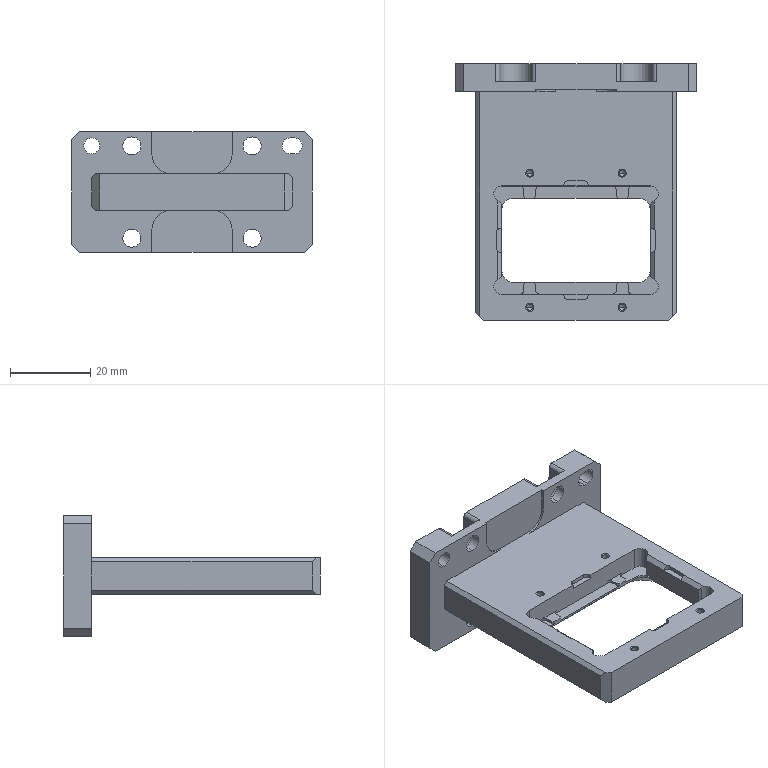NC program | NX | posted with a generic post | part box 60 x 64 x 30 mm
Whole program, first 2291 of 2766 lines:
N10 G17 G21 G94 G90
(FLOOR_WALL_COPY , TOOL : D20R0.8)
N12 T01 M6
N14 G54
N16 G17 G0 G90 X45. Y-29.999 B0. C0. S7500 M3
N18 G43 Z30. H1
N20 Z3.
N22 G94 G1 Z0. F1350.
N24 X42.
N26 X-42.
N28 Y-25.922
N30 Y-21.226
N32 X42.
N34 Y-12.453
N36 X-42.
N38 Y-3.68
N40 X42.
N42 Y5.094
N44 X-42.
N46 Y13.867
N48 X42.
N50 Y22.64
N52 X-42.
N54 X-45.
N56 Z3.
N58 G0 Z30.
N60 M5
(FLOOR_WALL_1_COPY_1 , TOOL : D10)
N62 T10 M6
N64 G54
N66 G17 G0 G90 X39.5 Y1.443 B0. C0. S9500 M3
N68 G43 Z30. H10
N70 Z1.153
N72 G94 G1 Z-0.347 F1000.
N74 X38.5 Y0.866
N76 G3 X38. Y0. R1.
N78 G1 Y-25.485 F3000.
N80 X33.485 Y-30.
N82 X-19.9
N84 Y-0.895
N86 X-20.4
N88 Y0.895
N90 X-19.9
N92 Y30.
N94 X33.485
N96 X38. Y25.485
N98 Y0.
N100 X32.
N102 Y-23.
N104 X31. Y-24.
N106 X-13.9
N108 Y-0.895
N110 G3 X-13.967 Y0. R6.
N112 X-13.9 Y0.895 R6.
N114 G1 Y24.
N116 X31.
N118 X32. Y23.
N120 Y0.
N122 X26.
N124 Y-18.
N126 X-7.9
N128 Y-0.895
N130 G3 X-7.933 Y0. R12.
N132 X-7.9 Y0.895 R12.
N134 G1 Y18.
N136 X26.
N138 Y0.
N140 X20.
N142 Y-12.
N144 X-1.9
N146 Y-0.895
N148 G3 X-1.922 Y0. R18.
N150 X-1.9 Y0.895 R18.
N152 G1 Y12.
N154 X20.
N156 Y0.
N158 X14.
N160 Y-6.
N162 X4.1
N164 Y-0.895
N166 G3 X4.083 Y0. R24.
N168 X4.1 Y0.895 R24.
N170 G1 Y6.
N172 X14.
N174 Y0.
N176 X9.5
N178 Y-1.5
N180 X8.6
N182 Y-0.895
N184 G3 X8.586 Y0. R28.5
N186 X8.6 Y0.895 R28.5
N188 G1 Y1.5
N190 X9.5
N192 Y0.
N194 G3 X10. Y-0.866 R1.
N196 G1 Z1.153
N198 G0 X39.5 Y1.443 Z0.807
N200 G1 Z-0.693 F1000.
N202 X38.5 Y0.866
N204 G3 X38. Y0. R1.
N206 G1 Y-25.485 F3000.
N208 X33.485 Y-30.
N210 X-19.9
N212 Y-0.895
N214 X-20.4
N216 Y0.895
N218 X-19.9
N220 Y30.
N222 X33.485
N224 X38. Y25.485
N226 Y0.
N228 X32.
N230 Y-23.
N232 X31. Y-24.
N234 X-13.9
N236 Y-0.895
N238 G3 X-13.967 Y0. R6.
N240 X-13.9 Y0.895 R6.
N242 G1 Y24.
N244 X31.
N246 X32. Y23.
N248 Y0.
N250 X26.
N252 Y-18.
N254 X-7.9
N256 Y-0.895
N258 G3 X-7.933 Y0. R12.
N260 X-7.9 Y0.895 R12.
N262 G1 Y18.
N264 X26.
N266 Y0.
N268 X20.
N270 Y-12.
N272 X-1.9
N274 Y-0.895
N276 G3 X-1.922 Y0. R18.
N278 X-1.9 Y0.895 R18.
N280 G1 Y12.
N282 X20.
N284 Y0.
N286 X14.
N288 Y-6.
N290 X4.1
N292 Y-0.895
N294 G3 X4.083 Y0. R24.
N296 X4.1 Y0.895 R24.
N298 G1 Y6.
N300 X14.
N302 Y0.
N304 X9.5
N306 Y-1.5
N308 X8.6
N310 Y-0.895
N312 G3 X8.586 Y0. R28.5
N314 X8.6 Y0.895 R28.5
N316 G1 Y1.5
N318 X9.5
N320 Y0.
N322 G3 X10. Y-0.866 R1.
N324 G1 Z0.807
N326 G0 X39.5 Y1.443 Z0.46
N328 G1 Z-1.04 F1000.
N330 X38.5 Y0.866
N332 G3 X38. Y0. R1.
N334 G1 Y-25.485 F3000.
N336 X33.485 Y-30.
N338 X-19.9
N340 Y-0.895
N342 X-20.4
N344 Y0.895
N346 X-19.9
N348 Y30.
N350 X33.485
N352 X38. Y25.485
N354 Y0.
N356 X32.
N358 Y-23.
N360 X31. Y-24.
N362 X-13.9
N364 Y-0.895
N366 G3 X-13.967 Y0. R6.
N368 X-13.9 Y0.895 R6.
N370 G1 Y24.
N372 X31.
N374 X32. Y23.
N376 Y0.
N378 X26.
N380 Y-18.
N382 X-7.9
N384 Y-0.895
N386 G3 X-7.933 Y0. R12.
N388 X-7.9 Y0.895 R12.
N390 G1 Y18.
N392 X26.
N394 Y0.
N396 X20.
N398 Y-12.
N400 X-1.9
N402 Y-0.895
N404 G3 X-1.922 Y0. R18.
N406 X-1.9 Y0.895 R18.
N408 G1 Y12.
N410 X20.
N412 Y0.
N414 X14.
N416 Y-6.
N418 X4.1
N420 Y-0.895
N422 G3 X4.083 Y0. R24.
N424 X4.1 Y0.895 R24.
N426 G1 Y6.
N428 X14.
N430 Y0.
N432 X9.5
N434 Y-1.5
N436 X8.6
N438 Y-0.895
N440 G3 X8.586 Y0. R28.5
N442 X8.6 Y0.895 R28.5
N444 G1 Y1.5
N446 X9.5
N448 Y0.
N450 G3 X10. Y-0.866 R1.
N452 G1 Z0.46
N454 G0 X39.5 Y1.443 Z0.113
N456 G1 Z-1.387 F1000.
N458 X38.5 Y0.866
N460 G3 X38. Y0. R1.
N462 G1 Y-25.485 F3000.
N464 X33.485 Y-30.
N466 X-19.9
N468 Y-0.895
N470 X-20.4
N472 Y0.895
N474 X-19.9
N476 Y30.
N478 X33.485
N480 X38. Y25.485
N482 Y0.
N484 X32.
N486 Y-23.
N488 X31. Y-24.
N490 X-13.9
N492 Y-0.895
N494 G3 X-13.967 Y0. R6.
N496 X-13.9 Y0.895 R6.
N498 G1 Y24.
N500 X31.
N502 X32. Y23.
N504 Y0.
N506 X26.
N508 Y-18.
N510 X-7.9
N512 Y-0.895
N514 G3 X-7.933 Y0. R12.
N516 X-7.9 Y0.895 R12.
N518 G1 Y18.
N520 X26.
N522 Y0.
N524 X20.
N526 Y-12.
N528 X-1.9
N530 Y-0.895
N532 G3 X-1.922 Y0. R18.
N534 X-1.9 Y0.895 R18.
N536 G1 Y12.
N538 X20.
N540 Y0.
N542 X14.
N544 Y-6.
N546 X4.1
N548 Y-0.895
N550 G3 X4.083 Y0. R24.
N552 X4.1 Y0.895 R24.
N554 G1 Y6.
N556 X14.
N558 Y0.
N560 X9.5
N562 Y-1.5
N564 X8.6
N566 Y-0.895
N568 G3 X8.586 Y0. R28.5
N570 X8.6 Y0.895 R28.5
N572 G1 Y1.5
N574 X9.5
N576 Y0.
N578 G3 X10. Y-0.866 R1.
N580 G1 Z0.113
N582 G0 X39.5 Y1.443 Z-0.233
N584 G1 Z-1.733 F1000.
N586 X38.5 Y0.866
N588 G3 X38. Y0. R1.
N590 G1 Y-25.485 F3000.
N592 X33.485 Y-30.
N594 X-19.9
N596 Y-0.895
N598 X-20.4
N600 Y0.895
N602 X-19.9
N604 Y30.
N606 X33.485
N608 X38. Y25.485
N610 Y0.
N612 X32.
N614 Y-23.
N616 X31. Y-24.
N618 X-13.9
N620 Y-0.895
N622 G3 X-13.967 Y0. R6.
N624 X-13.9 Y0.895 R6.
N626 G1 Y24.
N628 X31.
N630 X32. Y23.
N632 Y0.
N634 X26.
N636 Y-18.
N638 X-7.9
N640 Y-0.895
N642 G3 X-7.933 Y0. R12.
N644 X-7.9 Y0.895 R12.
N646 G1 Y18.
N648 X26.
N650 Y0.
N652 X20.
N654 Y-12.
N656 X-1.9
N658 Y-0.895
N660 G3 X-1.922 Y0. R18.
N662 X-1.9 Y0.895 R18.
N664 G1 Y12.
N666 X20.
N668 Y0.
N670 X14.
N672 Y-6.
N674 X4.1
N676 Y-0.895
N678 G3 X4.083 Y0. R24.
N680 X4.1 Y0.895 R24.
N682 G1 Y6.
N684 X14.
N686 Y0.
N688 X9.5
N690 Y-1.5
N692 X8.6
N694 Y-0.895
N696 G3 X8.586 Y0. R28.5
N698 X8.6 Y0.895 R28.5
N700 G1 Y1.5
N702 X9.5
N704 Y0.
N706 G3 X10. Y-0.866 R1.
N708 G1 Z-0.233
N710 G0 X39.5 Y1.443 Z-0.58
N712 G1 Z-2.08 F1000.
N714 X38.5 Y0.866
N716 G3 X38. Y0. R1.
N718 G1 Y-25.485 F3000.
N720 X33.485 Y-30.
N722 X-19.9
N724 Y-0.895
N726 X-20.4
N728 Y0.895
N730 X-19.9
N732 Y30.
N734 X33.485
N736 X38. Y25.485
N738 Y0.
N740 X32.
N742 Y-23.
N744 X31. Y-24.
N746 X-13.9
N748 Y-0.895
N750 G3 X-13.967 Y0. R6.
N752 X-13.9 Y0.895 R6.
N754 G1 Y24.
N756 X31.
N758 X32. Y23.
N760 Y0.
N762 X26.
N764 Y-18.
N766 X-7.9
N768 Y-0.895
N770 G3 X-7.933 Y0. R12.
N772 X-7.9 Y0.895 R12.
N774 G1 Y18.
N776 X26.
N778 Y0.
N780 X20.
N782 Y-12.
N784 X-1.9
N786 Y-0.895
N788 G3 X-1.922 Y0. R18.
N790 X-1.9 Y0.895 R18.
N792 G1 Y12.
N794 X20.
N796 Y0.
N798 X14.
N800 Y-6.
N802 X4.1
N804 Y-0.895
N806 G3 X4.083 Y0. R24.
N808 X4.1 Y0.895 R24.
N810 G1 Y6.
N812 X14.
N814 Y0.
N816 X9.5
N818 Y-1.5
N820 X8.6
N822 Y-0.895
N824 G3 X8.586 Y0. R28.5
N826 X8.6 Y0.895 R28.5
N828 G1 Y1.5
N830 X9.5
N832 Y0.
N834 G3 X10. Y-0.866 R1.
N836 G1 Z-0.58
N838 G0 X39.5 Y1.443 Z-0.927
N840 G1 Z-2.427 F1000.
N842 X38.5 Y0.866
N844 G3 X38. Y0. R1.
N846 G1 Y-25.485 F3000.
N848 X33.485 Y-30.
N850 X-19.9
N852 Y-0.895
N854 X-20.4
N856 Y0.895
N858 X-19.9
N860 Y30.
N862 X33.485
N864 X38. Y25.485
N866 Y0.
N868 X32.
N870 Y-23.
N872 X31. Y-24.
N874 X-13.9
N876 Y-0.895
N878 G3 X-13.967 Y0. R6.
N880 X-13.9 Y0.895 R6.
N882 G1 Y24.
N884 X31.
N886 X32. Y23.
N888 Y0.
N890 X26.
N892 Y-18.
N894 X-7.9
N896 Y-0.895
N898 G3 X-7.933 Y0. R12.
N900 X-7.9 Y0.895 R12.
N902 G1 Y18.
N904 X26.
N906 Y0.
N908 X20.
N910 Y-12.
N912 X-1.9
N914 Y-0.895
N916 G3 X-1.922 Y0. R18.
N918 X-1.9 Y0.895 R18.
N920 G1 Y12.
N922 X20.
N924 Y0.
N926 X14.
N928 Y-6.
N930 X4.1
N932 Y-0.895
N934 G3 X4.083 Y0. R24.
N936 X4.1 Y0.895 R24.
N938 G1 Y6.
N940 X14.
N942 Y0.
N944 X9.5
N946 Y-1.5
N948 X8.6
N950 Y-0.895
N952 G3 X8.586 Y0. R28.5
N954 X8.6 Y0.895 R28.5
N956 G1 Y1.5
N958 X9.5
N960 Y0.
N962 G3 X10. Y-0.866 R1.
N964 G1 Z-0.927
N966 G0 X39.5 Y1.443 Z-1.273
N968 G1 Z-2.773 F1000.
N970 X38.5 Y0.866
N972 G3 X38. Y0. R1.
N974 G1 Y-25.485 F3000.
N976 X33.485 Y-30.
N978 X-19.9
N980 Y-0.895
N982 X-20.4
N984 Y0.895
N986 X-19.9
N988 Y30.
N990 X33.485
N992 X38. Y25.485
N994 Y0.
N996 X32.
N998 Y-23.
N1000 X31. Y-24.
N1002 X-13.9
N1004 Y-0.895
N1006 G3 X-13.967 Y0. R6.
N1008 X-13.9 Y0.895 R6.
N1010 G1 Y24.
N1012 X31.
N1014 X32. Y23.
N1016 Y0.
N1018 X26.
N1020 Y-18.
N1022 X-7.9
N1024 Y-0.895
N1026 G3 X-7.933 Y0. R12.
N1028 X-7.9 Y0.895 R12.
N1030 G1 Y18.
N1032 X26.
N1034 Y0.
N1036 X20.
N1038 Y-12.
N1040 X-1.9
N1042 Y-0.895
N1044 G3 X-1.922 Y0. R18.
N1046 X-1.9 Y0.895 R18.
N1048 G1 Y12.
N1050 X20.
N1052 Y0.
N1054 X14.
N1056 Y-6.
N1058 X4.1
N1060 Y-0.895
N1062 G3 X4.083 Y0. R24.
N1064 X4.1 Y0.895 R24.
N1066 G1 Y6.
N1068 X14.
N1070 Y0.
N1072 X9.5
N1074 Y-1.5
N1076 X8.6
N1078 Y-0.895
N1080 G3 X8.586 Y0. R28.5
N1082 X8.6 Y0.895 R28.5
N1084 G1 Y1.5
N1086 X9.5
N1088 Y0.
N1090 G3 X10. Y-0.866 R1.
N1092 G1 Z-1.273
N1094 G0 X39.5 Y1.443 Z-1.62
N1096 G1 Z-3.12 F1000.
N1098 X38.5 Y0.866
N1100 G3 X38. Y0. R1.
N1102 G1 Y-25.485 F3000.
N1104 X33.485 Y-30.
N1106 X-19.9
N1108 Y-0.895
N1110 X-20.4
N1112 Y0.895
N1114 X-19.9
N1116 Y30.
N1118 X33.485
N1120 X38. Y25.485
N1122 Y0.
N1124 X32.
N1126 Y-23.
N1128 X31. Y-24.
N1130 X-13.9
N1132 Y-0.895
N1134 G3 X-13.967 Y0. R6.
N1136 X-13.9 Y0.895 R6.
N1138 G1 Y24.
N1140 X31.
N1142 X32. Y23.
N1144 Y0.
N1146 X26.
N1148 Y-18.
N1150 X-7.9
N1152 Y-0.895
N1154 G3 X-7.933 Y0. R12.
N1156 X-7.9 Y0.895 R12.
N1158 G1 Y18.
N1160 X26.
N1162 Y0.
N1164 X20.
N1166 Y-12.
N1168 X-1.9
N1170 Y-0.895
N1172 G3 X-1.922 Y0. R18.
N1174 X-1.9 Y0.895 R18.
N1176 G1 Y12.
N1178 X20.
N1180 Y0.
N1182 X14.
N1184 Y-6.
N1186 X4.1
N1188 Y-0.895
N1190 G3 X4.083 Y0. R24.
N1192 X4.1 Y0.895 R24.
N1194 G1 Y6.
N1196 X14.
N1198 Y0.
N1200 X9.5
N1202 Y-1.5
N1204 X8.6
N1206 Y-0.895
N1208 G3 X8.586 Y0. R28.5
N1210 X8.6 Y0.895 R28.5
N1212 G1 Y1.5
N1214 X9.5
N1216 Y0.
N1218 G3 X10. Y-0.866 R1.
N1220 G1 Z-1.62
N1222 G0 X39.5 Y1.443 Z-1.967
N1224 G1 Z-3.467 F1000.
N1226 X38.5 Y0.866
N1228 G3 X38. Y0. R1.
N1230 G1 Y-25.485 F3000.
N1232 X33.485 Y-30.
N1234 X-19.9
N1236 Y-0.895
N1238 X-20.4
N1240 Y0.895
N1242 X-19.9
N1244 Y30.
N1246 X33.485
N1248 X38. Y25.485
N1250 Y0.
N1252 X32.
N1254 Y-23.
N1256 X31. Y-24.
N1258 X-13.9
N1260 Y-0.895
N1262 G3 X-13.967 Y0. R6.
N1264 X-13.9 Y0.895 R6.
N1266 G1 Y24.
N1268 X31.
N1270 X32. Y23.
N1272 Y0.
N1274 X26.
N1276 Y-18.
N1278 X-7.9
N1280 Y-0.895
N1282 G3 X-7.933 Y0. R12.
N1284 X-7.9 Y0.895 R12.
N1286 G1 Y18.
N1288 X26.
N1290 Y0.
N1292 X20.
N1294 Y-12.
N1296 X-1.9
N1298 Y-0.895
N1300 G3 X-1.922 Y0. R18.
N1302 X-1.9 Y0.895 R18.
N1304 G1 Y12.
N1306 X20.
N1308 Y0.
N1310 X14.
N1312 Y-6.
N1314 X4.1
N1316 Y-0.895
N1318 G3 X4.083 Y0. R24.
N1320 X4.1 Y0.895 R24.
N1322 G1 Y6.
N1324 X14.
N1326 Y0.
N1328 X9.5
N1330 Y-1.5
N1332 X8.6
N1334 Y-0.895
N1336 G3 X8.586 Y0. R28.5
N1338 X8.6 Y0.895 R28.5
N1340 G1 Y1.5
N1342 X9.5
N1344 Y0.
N1346 G3 X10. Y-0.866 R1.
N1348 G1 Z-1.967
N1350 G0 X39.5 Y1.443 Z-2.313
N1352 G1 Z-3.813 F1000.
N1354 X38.5 Y0.866
N1356 G3 X38. Y0. R1.
N1358 G1 Y-25.485 F3000.
N1360 X33.485 Y-30.
N1362 X-19.9
N1364 Y-0.895
N1366 X-20.4
N1368 Y0.895
N1370 X-19.9
N1372 Y30.
N1374 X33.485
N1376 X38. Y25.485
N1378 Y0.
N1380 X32.
N1382 Y-23.
N1384 X31. Y-24.
N1386 X-13.9
N1388 Y-0.895
N1390 G3 X-13.967 Y0. R6.
N1392 X-13.9 Y0.895 R6.
N1394 G1 Y24.
N1396 X31.
N1398 X32. Y23.
N1400 Y0.
N1402 X26.
N1404 Y-18.
N1406 X-7.9
N1408 Y-0.895
N1410 G3 X-7.933 Y0. R12.
N1412 X-7.9 Y0.895 R12.
N1414 G1 Y18.
N1416 X26.
N1418 Y0.
N1420 X20.
N1422 Y-12.
N1424 X-1.9
N1426 Y-0.895
N1428 G3 X-1.922 Y0. R18.
N1430 X-1.9 Y0.895 R18.
N1432 G1 Y12.
N1434 X20.
N1436 Y0.
N1438 X14.
N1440 Y-6.
N1442 X4.1
N1444 Y-0.895
N1446 G3 X4.083 Y0. R24.
N1448 X4.1 Y0.895 R24.
N1450 G1 Y6.
N1452 X14.
N1454 Y0.
N1456 X9.5
N1458 Y-1.5
N1460 X8.6
N1462 Y-0.895
N1464 G3 X8.586 Y0. R28.5
N1466 X8.6 Y0.895 R28.5
N1468 G1 Y1.5
N1470 X9.5
N1472 Y0.
N1474 G3 X10. Y-0.866 R1.
N1476 G1 Z-2.313
N1478 G0 X39.5 Y1.443 Z-2.66
N1480 G1 Z-4.16 F1000.
N1482 X38.5 Y0.866
N1484 G3 X38. Y0. R1.
N1486 G1 Y-25.485 F3000.
N1488 X33.485 Y-30.
N1490 X-19.9
N1492 Y-0.895
N1494 X-20.4
N1496 Y0.895
N1498 X-19.9
N1500 Y30.
N1502 X33.485
N1504 X38. Y25.485
N1506 Y0.
N1508 X32.
N1510 Y-23.
N1512 X31. Y-24.
N1514 X-13.9
N1516 Y-0.895
N1518 G3 X-13.967 Y0. R6.
N1520 X-13.9 Y0.895 R6.
N1522 G1 Y24.
N1524 X31.
N1526 X32. Y23.
N1528 Y0.
N1530 X26.
N1532 Y-18.
N1534 X-7.9
N1536 Y-0.895
N1538 G3 X-7.933 Y0. R12.
N1540 X-7.9 Y0.895 R12.
N1542 G1 Y18.
N1544 X26.
N1546 Y0.
N1548 X20.
N1550 Y-12.
N1552 X-1.9
N1554 Y-0.895
N1556 G3 X-1.922 Y0. R18.
N1558 X-1.9 Y0.895 R18.
N1560 G1 Y12.
N1562 X20.
N1564 Y0.
N1566 X14.
N1568 Y-6.
N1570 X4.1
N1572 Y-0.895
N1574 G3 X4.083 Y0. R24.
N1576 X4.1 Y0.895 R24.
N1578 G1 Y6.
N1580 X14.
N1582 Y0.
N1584 X9.5
N1586 Y-1.5
N1588 X8.6
N1590 Y-0.895
N1592 G3 X8.586 Y0. R28.5
N1594 X8.6 Y0.895 R28.5
N1596 G1 Y1.5
N1598 X9.5
N1600 Y0.
N1602 G3 X10. Y-0.866 R1.
N1604 G1 Z-2.66
N1606 G0 X39.5 Y1.443 Z-3.007
N1608 G1 Z-4.507 F1000.
N1610 X38.5 Y0.866
N1612 G3 X38. Y0. R1.
N1614 G1 Y-25.485 F3000.
N1616 X33.485 Y-30.
N1618 X-19.9
N1620 Y-0.895
N1622 X-20.4
N1624 Y0.895
N1626 X-19.9
N1628 Y30.
N1630 X33.485
N1632 X38. Y25.485
N1634 Y0.
N1636 X32.
N1638 Y-23.
N1640 X31. Y-24.
N1642 X-13.9
N1644 Y-0.895
N1646 G3 X-13.967 Y0. R6.
N1648 X-13.9 Y0.895 R6.
N1650 G1 Y24.
N1652 X31.
N1654 X32. Y23.
N1656 Y0.
N1658 X26.
N1660 Y-18.
N1662 X-7.9
N1664 Y-0.895
N1666 G3 X-7.933 Y0. R12.
N1668 X-7.9 Y0.895 R12.
N1670 G1 Y18.
N1672 X26.
N1674 Y0.
N1676 X20.
N1678 Y-12.
N1680 X-1.9
N1682 Y-0.895
N1684 G3 X-1.922 Y0. R18.
N1686 X-1.9 Y0.895 R18.
N1688 G1 Y12.
N1690 X20.
N1692 Y0.
N1694 X14.
N1696 Y-6.
N1698 X4.1
N1700 Y-0.895
N1702 G3 X4.083 Y0. R24.
N1704 X4.1 Y0.895 R24.
N1706 G1 Y6.
N1708 X14.
N1710 Y0.
N1712 X9.5
N1714 Y-1.5
N1716 X8.6
N1718 Y-0.895
N1720 G3 X8.586 Y0. R28.5
N1722 X8.6 Y0.895 R28.5
N1724 G1 Y1.5
N1726 X9.5
N1728 Y0.
N1730 G3 X10. Y-0.866 R1.
N1732 G1 Z-3.007
N1734 G0 X39.5 Y1.443 Z-3.353
N1736 G1 Z-4.853 F1000.
N1738 X38.5 Y0.866
N1740 G3 X38. Y0. R1.
N1742 G1 Y-25.485 F3000.
N1744 X33.485 Y-30.
N1746 X-19.9
N1748 Y-0.895
N1750 X-20.4
N1752 Y0.895
N1754 X-19.9
N1756 Y30.
N1758 X33.485
N1760 X38. Y25.485
N1762 Y0.
N1764 X32.
N1766 Y-23.
N1768 X31. Y-24.
N1770 X-13.9
N1772 Y-0.895
N1774 G3 X-13.967 Y0. R6.
N1776 X-13.9 Y0.895 R6.
N1778 G1 Y24.
N1780 X31.
N1782 X32. Y23.
N1784 Y0.
N1786 X26.
N1788 Y-18.
N1790 X-7.9
N1792 Y-0.895
N1794 G3 X-7.933 Y0. R12.
N1796 X-7.9 Y0.895 R12.
N1798 G1 Y18.
N1800 X26.
N1802 Y0.
N1804 X20.
N1806 Y-12.
N1808 X-1.9
N1810 Y-0.895
N1812 G3 X-1.922 Y0. R18.
N1814 X-1.9 Y0.895 R18.
N1816 G1 Y12.
N1818 X20.
N1820 Y0.
N1822 X14.
N1824 Y-6.
N1826 X4.1
N1828 Y-0.895
N1830 G3 X4.083 Y0. R24.
N1832 X4.1 Y0.895 R24.
N1834 G1 Y6.
N1836 X14.
N1838 Y0.
N1840 X9.5
N1842 Y-1.5
N1844 X8.6
N1846 Y-0.895
N1848 G3 X8.586 Y0. R28.5
N1850 X8.6 Y0.895 R28.5
N1852 G1 Y1.5
N1854 X9.5
N1856 Y0.
N1858 G3 X10. Y-0.866 R1.
N1860 G1 Z-3.353
N1862 G0 X39.5 Y1.443 Z-3.7
N1864 G1 Z-5.2 F1000.
N1866 X38.5 Y0.866
N1868 G3 X38. Y0. R1.
N1870 G1 Y-25.485 F3000.
N1872 X33.485 Y-30.
N1874 X-19.9
N1876 Y-0.895
N1878 X-20.4
N1880 Y0.895
N1882 X-19.9
N1884 Y30.
N1886 X33.485
N1888 X38. Y25.485
N1890 Y0.
N1892 X32.
N1894 Y-23.
N1896 X31. Y-24.
N1898 X-13.9
N1900 Y-0.895
N1902 G3 X-13.967 Y0. R6.
N1904 X-13.9 Y0.895 R6.
N1906 G1 Y24.
N1908 X31.
N1910 X32. Y23.
N1912 Y0.
N1914 X26.
N1916 Y-18.
N1918 X-7.9
N1920 Y-0.895
N1922 G3 X-7.933 Y0. R12.
N1924 X-7.9 Y0.895 R12.
N1926 G1 Y18.
N1928 X26.
N1930 Y0.
N1932 X20.
N1934 Y-12.
N1936 X-1.9
N1938 Y-0.895
N1940 G3 X-1.922 Y0. R18.
N1942 X-1.9 Y0.895 R18.
N1944 G1 Y12.
N1946 X20.
N1948 Y0.
N1950 X14.
N1952 Y-6.
N1954 X4.1
N1956 Y-0.895
N1958 G3 X4.083 Y0. R24.
N1960 X4.1 Y0.895 R24.
N1962 G1 Y6.
N1964 X14.
N1966 Y0.
N1968 X9.5
N1970 Y-1.5
N1972 X8.6
N1974 Y-0.895
N1976 G3 X8.586 Y0. R28.5
N1978 X8.6 Y0.895 R28.5
N1980 G1 Y1.5
N1982 X9.5
N1984 Y0.
N1986 G3 X10. Y-0.866 R1.
N1988 G1 Z-3.7
N1990 G0 X39.5 Y1.443 Z-4.047
N1992 G1 Z-5.547 F1000.
N1994 X38.5 Y0.866
N1996 G3 X38. Y0. R1.
N1998 G1 Y-25.485 F3000.
N2000 X33.485 Y-30.
N2002 X-19.9
N2004 Y-0.895
N2006 X-20.4
N2008 Y0.895
N2010 X-19.9
N2012 Y30.
N2014 X33.485
N2016 X38. Y25.485
N2018 Y0.
N2020 X32.
N2022 Y-23.
N2024 X31. Y-24.
N2026 X-13.9
N2028 Y-0.895
N2030 G3 X-13.967 Y0. R6.
N2032 X-13.9 Y0.895 R6.
N2034 G1 Y24.
N2036 X31.
N2038 X32. Y23.
N2040 Y0.
N2042 X26.
N2044 Y-18.
N2046 X-7.9
N2048 Y-0.895
N2050 G3 X-7.933 Y0. R12.
N2052 X-7.9 Y0.895 R12.
N2054 G1 Y18.
N2056 X26.
N2058 Y0.
N2060 X20.
N2062 Y-12.
N2064 X-1.9
N2066 Y-0.895
N2068 G3 X-1.922 Y0. R18.
N2070 X-1.9 Y0.895 R18.
N2072 G1 Y12.
N2074 X20.
N2076 Y0.
N2078 X14.
N2080 Y-6.
N2082 X4.1
N2084 Y-0.895
N2086 G3 X4.083 Y0. R24.
N2088 X4.1 Y0.895 R24.
N2090 G1 Y6.
N2092 X14.
N2094 Y0.
N2096 X9.5
N2098 Y-1.5
N2100 X8.6
N2102 Y-0.895
N2104 G3 X8.586 Y0. R28.5
N2106 X8.6 Y0.895 R28.5
N2108 G1 Y1.5
N2110 X9.5
N2112 Y0.
N2114 G3 X10. Y-0.866 R1.
N2116 G1 Z-4.047
N2118 G0 X39.5 Y1.443 Z-4.393
N2120 G1 Z-5.893 F1000.
N2122 X38.5 Y0.866
N2124 G3 X38. Y0. R1.
N2126 G1 Y-25.485 F3000.
N2128 X33.485 Y-30.
N2130 X-19.9
N2132 Y-0.895
N2134 X-20.4
N2136 Y0.895
N2138 X-19.9
N2140 Y30.
N2142 X33.485
N2144 X38. Y25.485
N2146 Y0.
N2148 X32.
N2150 Y-23.
N2152 X31. Y-24.
N2154 X-13.9
N2156 Y-0.895
N2158 G3 X-13.967 Y0. R6.
N2160 X-13.9 Y0.895 R6.
N2162 G1 Y24.
N2164 X31.
N2166 X32. Y23.
N2168 Y0.
N2170 X26.
N2172 Y-18.
N2174 X-7.9
N2176 Y-0.895
N2178 G3 X-7.933 Y0. R12.
N2180 X-7.9 Y0.895 R12.
N2182 G1 Y18.
N2184 X26.
N2186 Y0.
N2188 X20.
N2190 Y-12.
N2192 X-1.9
N2194 Y-0.895
N2196 G3 X-1.922 Y0. R18.
N2198 X-1.9 Y0.895 R18.
N2200 G1 Y12.
N2202 X20.
N2204 Y0.
N2206 X14.
N2208 Y-6.
N2210 X4.1
N2212 Y-0.895
N2214 G3 X4.083 Y0. R24.
N2216 X4.1 Y0.895 R24.
N2218 G1 Y6.
N2220 X14.
N2222 Y0.
N2224 X9.5
N2226 Y-1.5
N2228 X8.6
N2230 Y-0.895
N2232 G3 X8.586 Y0. R28.5
N2234 X8.6 Y0.895 R28.5
N2236 G1 Y1.5
N2238 X9.5
N2240 Y0.
N2242 G3 X10. Y-0.866 R1.
N2244 G1 Z-4.393
N2246 G0 X39.5 Y1.443 Z-4.74
N2248 G1 Z-6.24 F1000.
N2250 X38.5 Y0.866
N2252 G3 X38. Y0. R1.
N2254 G1 Y-25.485 F3000.
N2256 X33.485 Y-30.
N2258 X-19.9
N2260 Y-0.895
N2262 X-20.4
N2264 Y0.895
N2266 X-19.9
N2268 Y30.
N2270 X33.485
N2272 X38. Y25.485
N2274 Y0.
N2276 X32.
N2278 Y-23.
N2280 X31. Y-24.
N2282 X-13.9
N2284 Y-0.895
N2286 G3 X-13.967 Y0. R6.
N2288 X-13.9 Y0.895 R6.
N2290 G1 Y24.
N2292 X31.
N2294 X32. Y23.
N2296 Y0.
N2298 X26.
N2300 Y-18.
N2302 X-7.9
N2304 Y-0.895
N2306 G3 X-7.933 Y0. R12.
N2308 X-7.9 Y0.895 R12.
N2310 G1 Y18.
N2312 X26.
N2314 Y0.
N2316 X20.
N2318 Y-12.
N2320 X-1.9
N2322 Y-0.895
N2324 G3 X-1.922 Y0. R18.
N2326 X-1.9 Y0.895 R18.
N2328 G1 Y12.
N2330 X20.
N2332 Y0.
N2334 X14.
N2336 Y-6.
N2338 X4.1
N2340 Y-0.895
N2342 G3 X4.083 Y0. R24.
N2344 X4.1 Y0.895 R24.
N2346 G1 Y6.
N2348 X14.
N2350 Y0.
N2352 X9.5
N2354 Y-1.5
N2356 X8.6
N2358 Y-0.895
N2360 G3 X8.586 Y0. R28.5
N2362 X8.6 Y0.895 R28.5
N2364 G1 Y1.5
N2366 X9.5
N2368 Y0.
N2370 G3 X10. Y-0.866 R1.
N2372 G1 Z-4.74
N2374 G0 X39.5 Y1.443 Z-5.087
N2376 G1 Z-6.587 F1000.
N2378 X38.5 Y0.866
N2380 G3 X38. Y0. R1.
N2382 G1 Y-25.485 F3000.
N2384 X33.485 Y-30.
N2386 X-19.9
N2388 Y-0.895
N2390 X-20.4
N2392 Y0.895
N2394 X-19.9
N2396 Y30.
N2398 X33.485
N2400 X38. Y25.485
N2402 Y0.
N2404 X32.
N2406 Y-23.
N2408 X31. Y-24.
N2410 X-13.9
N2412 Y-0.895
N2414 G3 X-13.967 Y0. R6.
N2416 X-13.9 Y0.895 R6.
N2418 G1 Y24.
N2420 X31.
N2422 X32. Y23.
N2424 Y0.
N2426 X26.
N2428 Y-18.
N2430 X-7.9
N2432 Y-0.895
N2434 G3 X-7.933 Y0. R12.
N2436 X-7.9 Y0.895 R12.
N2438 G1 Y18.
N2440 X26.
N2442 Y0.
N2444 X20.
N2446 Y-12.
N2448 X-1.9
N2450 Y-0.895
N2452 G3 X-1.922 Y0. R18.
N2454 X-1.9 Y0.895 R18.
N2456 G1 Y12.
N2458 X20.
N2460 Y0.
N2462 X14.
N2464 Y-6.
N2466 X4.1
N2468 Y-0.895
N2470 G3 X4.083 Y0. R24.
N2472 X4.1 Y0.895 R24.
N2474 G1 Y6.
N2476 X14.
N2478 Y0.
N2480 X9.5
N2482 Y-1.5
N2484 X8.6
N2486 Y-0.895
N2488 G3 X8.586 Y0. R28.5
N2490 X8.6 Y0.895 R28.5
N2492 G1 Y1.5
N2494 X9.5
N2496 Y0.
N2498 G3 X10. Y-0.866 R1.
N2500 G1 Z-5.087
N2502 G0 X39.5 Y1.443 Z-5.433
N2504 G1 Z-6.933 F1000.
N2506 X38.5 Y0.866
N2508 G3 X38. Y0. R1.
N2510 G1 Y-25.485 F3000.
N2512 X33.485 Y-30.
N2514 X-19.9
N2516 Y-0.895
N2518 X-20.4
N2520 Y0.895
N2522 X-19.9
N2524 Y30.
N2526 X33.485
N2528 X38. Y25.485
N2530 Y0.
N2532 X32.
N2534 Y-23.
N2536 X31. Y-24.
N2538 X-13.9
N2540 Y-0.895
N2542 G3 X-13.967 Y0. R6.
N2544 X-13.9 Y0.895 R6.
N2546 G1 Y24.
N2548 X31.
N2550 X32. Y23.
N2552 Y0.
N2554 X26.
N2556 Y-18.
N2558 X-7.9
N2560 Y-0.895
N2562 G3 X-7.933 Y0. R12.
N2564 X-7.9 Y0.895 R12.
N2566 G1 Y18.
N2568 X26.
N2570 Y0.
N2572 X20.
N2574 Y-12.
N2576 X-1.9
N2578 Y-0.895
N2580 G3 X-1.922 Y0. R18.
N2582 X-1.9 Y0.895 R18.
N2584 G1 Y12.
N2586 X20.
N2588 Y0.
N2590 X14.
N2592 Y-6.
N2594 X4.1
N2596 Y-0.895
N2598 G3 X4.083 Y0. R24.
N2600 X4.1 Y0.895 R24.
N2602 G1 Y6.
N2604 X14.
N2606 Y0.
N2608 X9.5
N2610 Y-1.5
N2612 X8.6
N2614 Y-0.895
N2616 G3 X8.586 Y0. R28.5
N2618 X8.6 Y0.895 R28.5
N2620 G1 Y1.5
N2622 X9.5
N2624 Y0.
N2626 G3 X10. Y-0.866 R1.
N2628 G1 Z-5.433
N2630 G0 X39.5 Y1.443 Z-5.78
N2632 G1 Z-7.28 F1000.
N2634 X38.5 Y0.866
N2636 G3 X38. Y0. R1.
N2638 G1 Y-25.485 F3000.
N2640 X33.485 Y-30.
N2642 X-19.9
N2644 Y-0.895
N2646 X-20.4
N2648 Y0.895
N2650 X-19.9
N2652 Y30.
N2654 X33.485
N2656 X38. Y25.485
N2658 Y0.
N2660 X32.
N2662 Y-23.
N2664 X31. Y-24.
N2666 X-13.9
N2668 Y-0.895
N2670 G3 X-13.967 Y0. R6.
N2672 X-13.9 Y0.895 R6.
N2674 G1 Y24.
N2676 X31.
N2678 X32. Y23.
N2680 Y0.
N2682 X26.
N2684 Y-18.
N2686 X-7.9
N2688 Y-0.895
N2690 G3 X-7.933 Y0. R12.
N2692 X-7.9 Y0.895 R12.
N2694 G1 Y18.
N2696 X26.
N2698 Y0.
N2700 X20.
N2702 Y-12.
N2704 X-1.9
N2706 Y-0.895
N2708 G3 X-1.922 Y0. R18.
N2710 X-1.9 Y0.895 R18.
N2712 G1 Y12.
N2714 X20.
N2716 Y0.
N2718 X14.
N2720 Y-6.
N2722 X4.1
N2724 Y-0.895
N2726 G3 X4.083 Y0. R24.
N2728 X4.1 Y0.895 R24.
N2730 G1 Y6.
N2732 X14.
N2734 Y0.
N2736 X9.5
N2738 Y-1.5
N2740 X8.6
N2742 Y-0.895
N2744 G3 X8.586 Y0. R28.5
N2746 X8.6 Y0.895 R28.5
N2748 G1 Y1.5
N2750 X9.5
N2752 Y0.
N2754 G3 X10. Y-0.866 R1.
N2756 G1 Z-5.78
N2758 G0 X39.5 Y1.443 Z-6.127
N2760 G1 Z-7.627 F1000.
N2762 X38.5 Y0.866
N2764 G3 X38. Y0. R1.
N2766 G1 Y-25.485 F3000.
N2768 X33.485 Y-30.
N2770 X-19.9
N2772 Y-0.895
N2774 X-20.4
N2776 Y0.895
N2778 X-19.9
N2780 Y30.
N2782 X33.485
N2784 X38. Y25.485
N2786 Y0.
N2788 X32.
N2790 Y-23.
N2792 X31. Y-24.
N2794 X-13.9
N2796 Y-0.895
N2798 G3 X-13.967 Y0. R6.
N2800 X-13.9 Y0.895 R6.
N2802 G1 Y24.
N2804 X31.
N2806 X32. Y23.
N2808 Y0.
N2810 X26.
N2812 Y-18.
N2814 X-7.9
N2816 Y-0.895
N2818 G3 X-7.933 Y0. R12.
N2820 X-7.9 Y0.895 R12.
N2822 G1 Y18.
N2824 X26.
N2826 Y0.
N2828 X20.
N2830 Y-12.
N2832 X-1.9
N2834 Y-0.895
N2836 G3 X-1.922 Y0. R18.
N2838 X-1.9 Y0.895 R18.
N2840 G1 Y12.
N2842 X20.
N2844 Y0.
N2846 X14.
N2848 Y-6.
N2850 X4.1
N2852 Y-0.895
N2854 G3 X4.083 Y0. R24.
N2856 X4.1 Y0.895 R24.
N2858 G1 Y6.
N2860 X14.
N2862 Y0.
N2864 X9.5
N2866 Y-1.5
N2868 X8.6
N2870 Y-0.895
N2872 G3 X8.586 Y0. R28.5
N2874 X8.6 Y0.895 R28.5
N2876 G1 Y1.5
N2878 X9.5
N2880 Y0.
N2882 G3 X10. Y-0.866 R1.
N2884 G1 Z-6.127
N2886 G0 X39.5 Y1.443 Z-6.473
N2888 G1 Z-7.973 F1000.
N2890 X38.5 Y0.866
N2892 G3 X38. Y0. R1.
N2894 G1 Y-25.485 F3000.
N2896 X33.485 Y-30.
N2898 X-19.9
N2900 Y-0.895
N2902 X-20.4
N2904 Y0.895
N2906 X-19.9
N2908 Y30.
N2910 X33.485
N2912 X38. Y25.485
N2914 Y0.
N2916 X32.
N2918 Y-23.
N2920 X31. Y-24.
N2922 X-13.9
N2924 Y-0.895
N2926 G3 X-13.967 Y0. R6.
N2928 X-13.9 Y0.895 R6.
N2930 G1 Y24.
N2932 X31.
N2934 X32. Y23.
N2936 Y0.
N2938 X26.
N2940 Y-18.
N2942 X-7.9
N2944 Y-0.895
N2946 G3 X-7.933 Y0. R12.
N2948 X-7.9 Y0.895 R12.
N2950 G1 Y18.
N2952 X26.
N2954 Y0.
N2956 X20.
N2958 Y-12.
N2960 X-1.9
N2962 Y-0.895
N2964 G3 X-1.922 Y0. R18.
N2966 X-1.9 Y0.895 R18.
N2968 G1 Y12.
N2970 X20.
N2972 Y0.
N2974 X14.
N2976 Y-6.
N2978 X4.1
N2980 Y-0.895
N2982 G3 X4.083 Y0. R24.
N2984 X4.1 Y0.895 R24.
N2986 G1 Y6.
N2988 X14.
N2990 Y0.
N2992 X9.5
N2994 Y-1.5
N2996 X8.6
N2998 Y-0.895
N3000 G3 X8.586 Y0. R28.5
N3002 X8.6 Y0.895 R28.5
N3004 G1 Y1.5
N3006 X9.5
N3008 Y0.
N3010 G3 X10. Y-0.866 R1.
N3012 G1 Z-6.473
N3014 G0 X39.5 Y1.443 Z-6.82
N3016 G1 Z-8.32 F1000.
N3018 X38.5 Y0.866
N3020 G3 X38. Y0. R1.
N3022 G1 Y-25.485 F3000.
N3024 X33.485 Y-30.
N3026 X-19.9
N3028 Y-0.895
N3030 X-20.4
N3032 Y0.895
N3034 X-19.9
N3036 Y30.
N3038 X33.485
N3040 X38. Y25.485
N3042 Y0.
N3044 X32.
N3046 Y-23.
N3048 X31. Y-24.
N3050 X-13.9
N3052 Y-0.895
N3054 G3 X-13.967 Y0. R6.
N3056 X-13.9 Y0.895 R6.
N3058 G1 Y24.
N3060 X31.
N3062 X32. Y23.
N3064 Y0.
N3066 X26.
N3068 Y-18.
N3070 X-7.9
N3072 Y-0.895
N3074 G3 X-7.933 Y0. R12.
N3076 X-7.9 Y0.895 R12.
N3078 G1 Y18.
N3080 X26.
N3082 Y0.
N3084 X20.
N3086 Y-12.
N3088 X-1.9
N3090 Y-0.895
N3092 G3 X-1.922 Y0. R18.
N3094 X-1.9 Y0.895 R18.
N3096 G1 Y12.
N3098 X20.
N3100 Y0.
N3102 X14.
N3104 Y-6.
N3106 X4.1
N3108 Y-0.895
N3110 G3 X4.083 Y0. R24.
N3112 X4.1 Y0.895 R24.
N3114 G1 Y6.
N3116 X14.
N3118 Y0.
N3120 X9.5
N3122 Y-1.5
N3124 X8.6
N3126 Y-0.895
N3128 G3 X8.586 Y0. R28.5
N3130 X8.6 Y0.895 R28.5
N3132 G1 Y1.5
N3134 X9.5
N3136 Y0.
N3138 G3 X10. Y-0.866 R1.
N3140 G1 Z-6.82
N3142 G0 X39.5 Y1.443 Z-7.167
N3144 G1 Z-8.667 F1000.
N3146 X38.5 Y0.866
N3148 G3 X38. Y0. R1.
N3150 G1 Y-25.485 F3000.
N3152 X33.485 Y-30.
N3154 X-19.9
N3156 Y-0.895
N3158 X-20.4
N3160 Y0.895
N3162 X-19.9
N3164 Y30.
N3166 X33.485
N3168 X38. Y25.485
N3170 Y0.
N3172 X32.
N3174 Y-23.
N3176 X31. Y-24.
N3178 X-13.9
N3180 Y-0.895
N3182 G3 X-13.967 Y0. R6.
N3184 X-13.9 Y0.895 R6.
N3186 G1 Y24.
N3188 X31.
N3190 X32. Y23.
N3192 Y0.
N3194 X26.
N3196 Y-18.
N3198 X-7.9
N3200 Y-0.895
N3202 G3 X-7.933 Y0. R12.
N3204 X-7.9 Y0.895 R12.
N3206 G1 Y18.
N3208 X26.
N3210 Y0.
N3212 X20.
N3214 Y-12.
N3216 X-1.9
N3218 Y-0.895
N3220 G3 X-1.922 Y0. R18.
N3222 X-1.9 Y0.895 R18.
N3224 G1 Y12.
N3226 X20.
N3228 Y0.
N3230 X14.
N3232 Y-6.
N3234 X4.1
N3236 Y-0.895
N3238 G3 X4.083 Y0. R24.
N3240 X4.1 Y0.895 R24.
N3242 G1 Y6.
N3244 X14.
N3246 Y0.
N3248 X9.5
N3250 Y-1.5
N3252 X8.6
N3254 Y-0.895
N3256 G3 X8.586 Y0. R28.5
N3258 X8.6 Y0.895 R28.5
N3260 G1 Y1.5
N3262 X9.5
N3264 Y0.
N3266 G3 X10. Y-0.866 R1.
N3268 G1 Z-7.167
N3270 G0 X39.5 Y1.443 Z-7.513
N3272 G1 Z-9.013 F1000.
N3274 X38.5 Y0.866
N3276 G3 X38. Y0. R1.
N3278 G1 Y-25.485 F3000.
N3280 X33.485 Y-30.
N3282 X-19.9
N3284 Y-0.895
N3286 X-20.4
N3288 Y0.895
N3290 X-19.9
N3292 Y30.
N3294 X33.485
N3296 X38. Y25.485
N3298 Y0.
N3300 X32.
N3302 Y-23.
N3304 X31. Y-24.
N3306 X-13.9
N3308 Y-0.895
N3310 G3 X-13.967 Y0. R6.
N3312 X-13.9 Y0.895 R6.
N3314 G1 Y24.
N3316 X31.
N3318 X32. Y23.
N3320 Y0.
N3322 X26.
N3324 Y-18.
N3326 X-7.9
N3328 Y-0.895
N3330 G3 X-7.933 Y0. R12.
N3332 X-7.9 Y0.895 R12.
N3334 G1 Y18.
N3336 X26.
N3338 Y0.
N3340 X20.
N3342 Y-12.
N3344 X-1.9
N3346 Y-0.895
N3348 G3 X-1.922 Y0. R18.
N3350 X-1.9 Y0.895 R18.
N3352 G1 Y12.
N3354 X20.
N3356 Y0.
N3358 X14.
N3360 Y-6.
N3362 X4.1
N3364 Y-0.895
N3366 G3 X4.083 Y0. R24.
N3368 X4.1 Y0.895 R24.
N3370 G1 Y6.
N3372 X14.
N3374 Y0.
N3376 X9.5
N3378 Y-1.5
N3380 X8.6
N3382 Y-0.895
N3384 G3 X8.586 Y0. R28.5
N3386 X8.6 Y0.895 R28.5
N3388 G1 Y1.5
N3390 X9.5
N3392 Y0.
N3394 G3 X10. Y-0.866 R1.
N3396 G1 Z-7.513
N3398 G0 X39.5 Y1.443 Z-7.86
N3400 G1 Z-9.36 F1000.
N3402 X38.5 Y0.866
N3404 G3 X38. Y0. R1.
N3406 G1 Y-25.485 F3000.
N3408 X33.485 Y-30.
N3410 X-19.9
N3412 Y-0.895
N3414 X-20.4
N3416 Y0.895
N3418 X-19.9
N3420 Y30.
N3422 X33.485
N3424 X38. Y25.485
N3426 Y0.
N3428 X32.
N3430 Y-23.
N3432 X31. Y-24.
N3434 X-13.9
N3436 Y-0.895
N3438 G3 X-13.967 Y0. R6.
N3440 X-13.9 Y0.895 R6.
N3442 G1 Y24.
N3444 X31.
N3446 X32. Y23.
N3448 Y0.
N3450 X26.
N3452 Y-18.
N3454 X-7.9
N3456 Y-0.895
N3458 G3 X-7.933 Y0. R12.
N3460 X-7.9 Y0.895 R12.
N3462 G1 Y18.
N3464 X26.
N3466 Y0.
N3468 X20.
N3470 Y-12.
N3472 X-1.9
N3474 Y-0.895
N3476 G3 X-1.922 Y0. R18.
N3478 X-1.9 Y0.895 R18.
N3480 G1 Y12.
N3482 X20.
N3484 Y0.
N3486 X14.
N3488 Y-6.
N3490 X4.1
N3492 Y-0.895
N3494 G3 X4.083 Y0. R24.
N3496 X4.1 Y0.895 R24.
N3498 G1 Y6.
N3500 X14.
N3502 Y0.
N3504 X9.5
N3506 Y-1.5
N3508 X8.6
N3510 Y-0.895
N3512 G3 X8.586 Y0. R28.5
N3514 X8.6 Y0.895 R28.5
N3516 G1 Y1.5
N3518 X9.5
N3520 Y0.
N3522 G3 X10. Y-0.866 R1.
N3524 G1 Z-7.86
N3526 G0 X39.5 Y1.443 Z-8.207
N3528 G1 Z-9.707 F1000.
N3530 X38.5 Y0.866
N3532 G3 X38. Y0. R1.
N3534 G1 Y-25.485 F3000.
N3536 X33.485 Y-30.
N3538 X-19.9
N3540 Y-0.895
N3542 X-20.4
N3544 Y0.895
N3546 X-19.9
N3548 Y30.
N3550 X33.485
N3552 X38. Y25.485
N3554 Y0.
N3556 X32.
N3558 Y-23.
N3560 X31. Y-24.
N3562 X-13.9
N3564 Y-0.895
N3566 G3 X-13.967 Y0. R6.
N3568 X-13.9 Y0.895 R6.
N3570 G1 Y24.
N3572 X31.
N3574 X32. Y23.
N3576 Y0.
N3578 X26.
N3580 Y-18.
N3582 X-7.9
N3584 Y-0.895
N3586 G3 X-7.933 Y0. R12.
N3588 X-7.9 Y0.895 R12.
N3590 G1 Y18.
N3592 X26.
N3594 Y0.
N3596 X20.
N3598 Y-12.
N3600 X-1.9
N3602 Y-0.895
N3604 G3 X-1.922 Y0. R18.
N3606 X-1.9 Y0.895 R18.
N3608 G1 Y12.
N3610 X20.
N3612 Y0.
N3614 X14.
N3616 Y-6.
N3618 X4.1
N3620 Y-0.895
N3622 G3 X4.083 Y0. R24.
N3624 X4.1 Y0.895 R24.
N3626 G1 Y6.
N3628 X14.
N3630 Y0.
N3632 X9.5
N3634 Y-1.5
N3636 X8.6
N3638 Y-0.895
N3640 G3 X8.586 Y0. R28.5
N3642 X8.6 Y0.895 R28.5
N3644 G1 Y1.5
N3646 X9.5
N3648 Y0.
N3650 G3 X10. Y-0.866 R1.
N3652 G1 Z-8.207
N3654 G0 X39.5 Y1.443 Z-8.553
N3656 G1 Z-10.053 F1000.
N3658 X38.5 Y0.866
N3660 G3 X38. Y0. R1.
N3662 G1 Y-25.485 F3000.
N3664 X33.485 Y-30.
N3666 X-19.9
N3668 Y-0.895
N3670 X-20.4
N3672 Y0.895
N3674 X-19.9
N3676 Y30.
N3678 X33.485
N3680 X38. Y25.485
N3682 Y0.
N3684 X32.
N3686 Y-23.
N3688 X31. Y-24.
N3690 X-13.9
N3692 Y-0.895
N3694 G3 X-13.967 Y0. R6.
N3696 X-13.9 Y0.895 R6.
N3698 G1 Y24.
N3700 X31.
N3702 X32. Y23.
N3704 Y0.
N3706 X26.
N3708 Y-18.
N3710 X-7.9
N3712 Y-0.895
N3714 G3 X-7.933 Y0. R12.
N3716 X-7.9 Y0.895 R12.
N3718 G1 Y18.
N3720 X26.
N3722 Y0.
N3724 X20.
N3726 Y-12.
N3728 X-1.9
N3730 Y-0.895
N3732 G3 X-1.922 Y0. R18.
N3734 X-1.9 Y0.895 R18.
N3736 G1 Y12.
N3738 X20.
N3740 Y0.
N3742 X14.
N3744 Y-6.
N3746 X4.1
N3748 Y-0.895
N3750 G3 X4.083 Y0. R24.
N3752 X4.1 Y0.895 R24.
N3754 G1 Y6.
N3756 X14.
N3758 Y0.
N3760 X9.5
N3762 Y-1.5
N3764 X8.6
N3766 Y-0.895
N3768 G3 X8.586 Y0. R28.5
N3770 X8.6 Y0.895 R28.5
N3772 G1 Y1.5
N3774 X9.5
N3776 Y0.
N3778 G3 X10. Y-0.866 R1.
N3780 G1 Z-8.553
N3782 G0 X39.5 Y1.443 Z-8.9
N3784 G1 Z-10.4 F1000.
N3786 X38.5 Y0.866
N3788 G3 X38. Y0. R1.
N3790 G1 Y-25.485 F3000.
N3792 X33.485 Y-30.
N3794 X-19.9
N3796 Y-0.895
N3798 X-20.4
N3800 Y0.895
N3802 X-19.9
N3804 Y30.
N3806 X33.485
N3808 X38. Y25.485
N3810 Y0.
N3812 X32.
N3814 Y-23.
N3816 X31. Y-24.
N3818 X-13.9
N3820 Y-0.895
N3822 G3 X-13.967 Y0. R6.
N3824 X-13.9 Y0.895 R6.
N3826 G1 Y24.
N3828 X31.
N3830 X32. Y23.
N3832 Y0.
N3834 X26.
N3836 Y-18.
N3838 X-7.9
N3840 Y-0.895
N3842 G3 X-7.933 Y0. R12.
N3844 X-7.9 Y0.895 R12.
N3846 G1 Y18.
N3848 X26.
N3850 Y0.
N3852 X20.
N3854 Y-12.
N3856 X-1.9
N3858 Y-0.895
N3860 G3 X-1.922 Y0. R18.
N3862 X-1.9 Y0.895 R18.
N3864 G1 Y12.
N3866 X20.
N3868 Y0.
N3870 X14.
N3872 Y-6.
N3874 X4.1
N3876 Y-0.895
N3878 G3 X4.083 Y0. R24.
N3880 X4.1 Y0.895 R24.
N3882 G1 Y6.
N3884 X14.
N3886 Y0.
N3888 X9.5
N3890 Y-1.5
N3892 X8.6
N3894 Y-0.895
N3896 G3 X8.586 Y0. R28.5
N3898 X8.6 Y0.895 R28.5
N3900 G1 Y1.5
N3902 X9.5
N3904 Y0.
N3906 G3 X10. Y-0.866 R1.
N3908 G1 Z-8.9
N3910 G0 Z30.
(ZLEVEL_PROFILE_COPY_1_COPY_COPY , TOOL : D4R0.5)
N3912 T05 M6
N3914 G17 G43 G0 G90 X-22.531 Y8.918 Z30. B0. C0. S9500 H5 M3
N3916 Z0.8
N3918 G94 G1 Z-0.2 F2500.
N3920 X-23.132 Y8.99
N3922 G3 X-23.499 Y8.832 R0.4
N3924 G1 X-23.5 Y8.669
N3926 Y-8.
N3928 X-23.497 Y-8.84
N3930 X-23.481 Y-8.767 Z-0.3
N3932 X-23.497 Y-8.696 Z-0.4
N3934 X-23.499 Y-8.674
N3936 X-23.5 Y-8.
N3938 Y8.695
N3940 X-23.466 Y8.717 Z-0.6
N3942 X-23.5 Y8.684
N3944 Y-8.684
N3946 X-23.467 Y-8.715
N3948 Z-0.8
N3950 X-23.5 Y-8.684
N3952 Y8.684
N3954 X-23.466 Y8.717
N3956 Z-1.
N3958 X-23.5 Y8.683
N3960 Y-8.684
N3962 X-23.474 Y-8.708
N3964 Z-1.2
N3966 X-23.5 Y-8.674
N3968 Y8.683
N3970 X-23.466 Y8.717
N3972 Z-1.4
N3974 X-23.5 Y8.683
N3976 Y-8.674
N3978 X-23.474 Y-8.708
N3980 X-23.473 Z-1.6
N3982 X-23.5 Y-8.674
N3984 Y8.683
N3986 X-23.466 Y8.717
N3988 Z-1.8
N3990 X-23.5 Y8.683
N3992 Y-8.674
N3994 X-23.473 Y-8.708
N3996 Z-2.
N3998 X-23.5 Y-8.674
N4000 Y8.683
N4002 X-23.466 Y8.717
N4004 Z-2.2
N4006 X-23.5 Y8.683
N4008 Y-8.674
N4010 X-23.473 Y-8.708
N4012 Z-2.4
N4014 X-23.5 Y-8.674
N4016 Y8.683
N4018 X-23.466 Y8.717
N4020 Z-2.6
N4022 X-23.5 Y8.683
N4024 Y-8.674
N4026 X-23.473 Y-8.709
N4028 Z-2.8
N4030 X-23.5 Y-8.674
N4032 Y8.683
N4034 X-23.466 Y8.717
N4036 Z-3.
N4038 X-23.5 Y8.683
N4040 Y-8.674
N4042 X-23.473 Y-8.709
N4044 Z-3.2
N4046 X-23.5 Y-8.674
N4048 Y8.683
N4050 X-23.466 Y8.717
N4052 Z-3.4
N4054 X-23.5 Y8.682
N4056 Y-8.674
N4058 X-23.472 Y-8.709
N4060 Z-3.6
N4062 X-23.5 Y-8.674
N4064 Y8.682
N4066 X-23.466 Y8.717
N4068 X-23.475 Y8.706 Z-3.8
N4070 X-23.5 Y8.682
N4072 Y-8.674
N4074 X-23.472 Y-8.709
N4076 Z-4.
N4078 X-23.5 Y-8.674
N4080 Y8.682
N4082 X-23.475 Y8.706
N4084 Z-4.2
N4086 X-23.5 Y8.682
N4088 Y-8.674
N4090 X-23.472 Y-8.71
N4092 Z-4.4
N4094 X-23.5 Y-8.674
N4096 Y8.682
N4098 X-23.475 Y8.706
N4100 Z-4.6
N4102 X-23.5 Y8.682
N4104 Y-8.674
N4106 X-23.472 Y-8.71
N4108 Z-4.8
N4110 X-23.5 Y-8.674
N4112 Y8.682
N4114 X-23.475 Y8.706
N4116 Z-5.
N4118 X-23.5 Y8.682
N4120 Y-8.674
N4122 X-23.472 Y-8.71
N4124 X-23.471 Z-5.2
N4126 X-23.5 Y-8.674
N4128 Y8.682
N4130 X-23.475 Y8.707
N4132 X-23.474 Z-5.4
N4134 X-23.5 Y8.682
N4136 Y-8.674
N4138 X-23.471 Y-8.71
N4140 Y-8.711 Z-5.6
N4142 X-23.5 Y-8.674
N4144 Y8.681
N4146 X-23.474 Y8.707
N4148 Z-5.8
N4150 X-23.5 Y8.681
N4152 Y-8.674
N4154 X-23.471 Y-8.711
N4156 Z-6.
N4158 X-23.5 Y-8.674
N4160 Y8.681
N4162 X-23.474 Y8.707
N4164 X-23.5 Y8.669 Z-6.2
N4166 Y-8.674
N4168 Y-8.661 Z-6.4
N4170 Y8.656
N4172 Y8.64 Z-6.6
N4174 Y-8.64
N4176 Y-8.604 Z-6.8
N4178 Y8.599
N4180 Y8.561 Z-7.
N4182 Y-8.56
N4184 Y-8.515 Z-7.2
N4186 Y8.514
N4188 Y8.45 Z-7.4
N4190 Y-8.45
N4192 Y-8.387 Z-7.6
N4194 Y8.386
N4196 Y8.307 Z-7.8
N4198 Y-8.308
N4200 Y-8.215 Z-8.
N4202 Y8.216
N4204 Y8.109 Z-8.2
N4206 Y-8.122
N4208 Y-8.001 Z-8.4
N4210 Y8.
N4212 Y7.875 Z-8.6
N4214 Y-7.876
N4216 Y-7.733 Z-8.8
N4218 Y7.732
N4220 Y7.565 Z-9.
N4222 Y-7.565
N4224 Y-7.39 Z-9.2
N4226 Y7.39
N4228 Y7.184 Z-9.4
N4230 Y-7.173
N4232 Y-6.927 Z-9.6
N4234 Y6.927
N4236 Y6.667 Z-9.8
N4238 Y-6.667
N4240 Y-6.375 Z-9.975
N4242 Y6.375
N4244 Y6.037 Z-10.15
N4246 Y-6.037
N4248 Y-5.601 Z-10.325
N4250 Y5.601
N4252 Y4.756 Z-10.5
N4254 Y-4.756
N4256 G3 X-23.186 Y-5.004 R0.4
N4258 G1 X-22.533 Y-5.097
N4260 Z-9.5
N4262 G0 Z30.
(ZLEVEL_PROFILE_COPY_1_COPY_COPY_COPY_COPY , TOOL : D4R0.5)
N4264 X22.92 Y-0.693
N4266 Z-9.571
N4268 G1 Z-10.571
N4270 X23.52 Y-0.346
N4272 G3 X23.72 Y0. R0.4
N4274 G1 X23.722 Y15.224
N4276 X23.715 Y15.506
N4278 G3 X19.485 Y19.715 R4.234
N4280 G1 X19.203 Y19.718
N4282 X4.797 Y19.722
N4284 X4.515 Y19.717
N4286 G3 X0.287 Y15.506 R4.235
N4288 G1 X0.282 Y15.224
N4290 X0.278 Y-15.224
N4292 X0.285 Y-15.506
N4294 G3 X4.515 Y-19.715 R4.235
N4296 G1 X4.797 Y-19.718
N4298 X19.203 Y-19.722
N4300 X19.485 Y-19.717
N4302 G3 X23.713 Y-15.506 R4.234
N4304 G1 X23.718 Y-15.224
N4306 X23.72 Y0.
N4308 X23.687 Z-10.606
N4310 X23.651 Z-10.641
N4312 Y-15.224
N4314 X23.647 Y-15.506
N4316 G2 X19.485 Y-19.649 R4.164
N4318 G1 X19.203 Y-19.651
N4320 X4.797
N4322 X4.515 Y-19.649
N4324 G2 X0.352 Y-15.506 R4.164
N4326 G1 X0.349 Y-15.224
N4328 Y15.224
N4330 X0.353 Y15.506
N4332 G2 X4.515 Y19.649 R4.164
N4334 G1 X4.797 Y19.651
N4336 X19.203
N4338 X19.485 Y19.649
N4340 G2 X23.648 Y15.506 R4.164
N4342 G1 X23.651 Y15.224
N4344 Y0.
N4346 X23.616 Z-10.677
N4348 X23.581 Z-10.712
N4350 Y15.5
N4352 G3 X19.5 Y19.581 R4.081
N4354 G1 X4.5
N4356 G3 X0.419 Y15.5 R4.081
N4358 G1 Y-15.5
N4360 G3 X4.5 Y-19.581 R4.081
N4362 G1 X19.5
N4364 G3 X23.581 Y-15.5 R4.081
N4366 G1 Y0.
N4368 X23.51 Z-10.783
N4370 Y-15.5
N4372 G2 X19.5 Y-19.51 R4.01
N4374 G1 X4.5
N4376 G2 X0.49 Y-15.5 R4.01
N4378 G1 Y15.5
N4380 G2 X4.5 Y19.51 R4.01
N4382 G1 X19.5
N4384 G2 X23.51 Y15.5 R4.01
N4386 G1 Y0.
N4388 X23.439 Z-10.854
N4390 Y15.5
N4392 G3 X19.5 Y19.439 R3.939
N4394 G1 X4.5
N4396 G3 X0.561 Y15.5 R3.939
N4398 G1 Y-15.5
N4400 G3 X4.5 Y-19.439 R3.939
N4402 G1 X19.5
N4404 G3 X23.439 Y-15.5 R3.939
N4406 G1 Y0.
N4408 X23.369 Z-10.924
N4410 Y-15.5
N4412 G2 X19.5 Y-19.369 R3.869
N4414 G1 X4.5
N4416 G2 X0.631 Y-15.5 R3.869
N4418 G1 Y15.5
N4420 G2 X4.5 Y19.369 R3.869
N4422 G1 X19.5
N4424 G2 X23.369 Y15.5 R3.869
N4426 G1 Y0.
N4428 X23.298 Z-10.995
N4430 Y15.5
N4432 G3 X19.5 Y19.298 R3.798
N4434 G1 X4.5
N4436 G3 X0.702 Y15.5 R3.798
N4438 G1 Y-15.5
N4440 G3 X4.5 Y-19.298 R3.798
N4442 G1 X19.5
N4444 G3 X23.298 Y-15.5 R3.798
N4446 G1 Y0.
N4448 X23.227 Z-11.066
N4450 Y-15.5
N4452 G2 X19.5 Y-19.227 R3.727
N4454 G1 X4.5
N4456 G2 X0.773 Y-15.5 R3.727
N4458 G1 Y15.5
N4460 G2 X4.5 Y19.227 R3.727
N4462 G1 X19.5
N4464 G2 X23.227 Y15.5 R3.727
N4466 G1 Y0.
N4468 X23.156 Z-11.136
N4470 Y15.5
N4472 G3 X19.5 Y19.156 R3.656
N4474 G1 X4.5
N4476 G3 X0.844 Y15.5 R3.656
N4478 G1 Y-15.5
N4480 G3 X4.5 Y-19.156 R3.656
N4482 G1 X19.5
N4484 G3 X23.156 Y-15.5 R3.656
N4486 G1 Y0.
N4488 X23.086 Z-11.207
N4490 Y-15.5
N4492 G2 X19.5 Y-19.086 R3.586
N4494 G1 X4.5
N4496 G2 X0.914 Y-15.5 R3.586
N4498 G1 Y15.5
N4500 G2 X4.5 Y19.086 R3.586
N4502 G1 X19.5
N4504 G2 X23.086 Y15.5 R3.586
N4506 G1 Y0.
N4508 X23.015 Z-11.278
N4510 Y15.5
N4512 G3 X19.5 Y19.015 R3.515
N4514 G1 X4.5
N4516 G3 X0.985 Y15.5 R3.515
N4518 G1 Y-15.5
N4520 G3 X4.5 Y-19.015 R3.515
N4522 G1 X19.5
N4524 G3 X23.015 Y-15.5 R3.515
N4526 G1 Y0.
N4528 X22.944 Z-11.349
N4530 Y-15.5
N4532 G2 X19.5 Y-18.944 R3.444
N4534 G1 X4.5
N4536 G2 X1.056 Y-15.5 R3.444
N4538 G1 Y15.5
N4540 G2 X4.5 Y18.944 R3.444
N4542 G1 X19.5
N4544 G2 X22.944 Y15.5 R3.444
N4546 G1 Y0.
N4548 X22.874 Z-11.419
N4550 Y15.5
N4552 G3 X19.5 Y18.874 R3.374
N4554 G1 X4.5
N4556 G3 X1.126 Y15.5 R3.374
N4558 G1 Y-15.5
N4560 G3 X4.5 Y-18.874 R3.374
N4562 G1 X19.5
N4564 G3 X22.874 Y-15.5 R3.374
N4566 G1 Y0.
N4568 X22.803 Z-11.49
N4570 Y-15.5
N4572 G2 X19.5 Y-18.803 R3.303
N4574 G1 X4.5
N4576 G2 X1.197 Y-15.5 R3.303
N4578 G1 Y15.5
N4580 G2 X4.5 Y18.803 R3.303
N4582 G1 X19.5